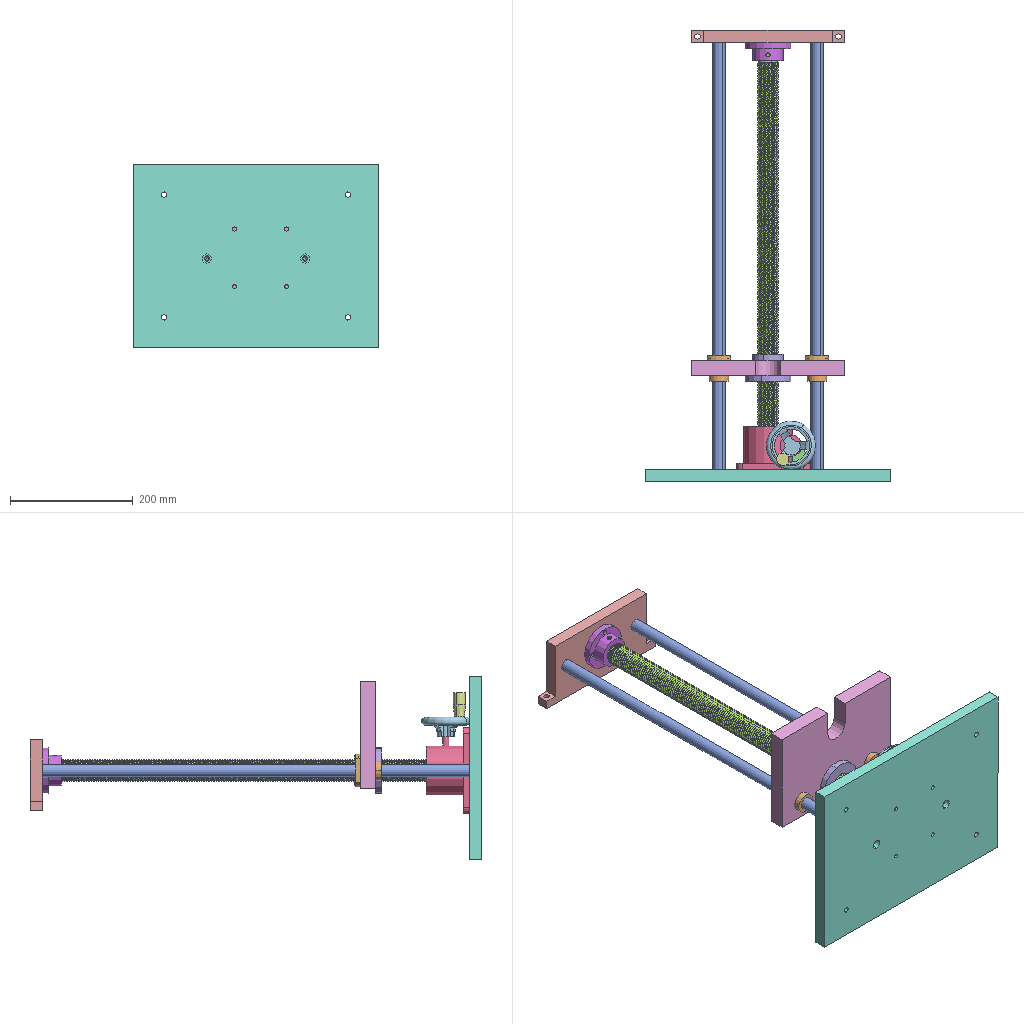Assembly | SolidWorks | 12 different items | 14 placed | box 400 x 736 x 300 mm
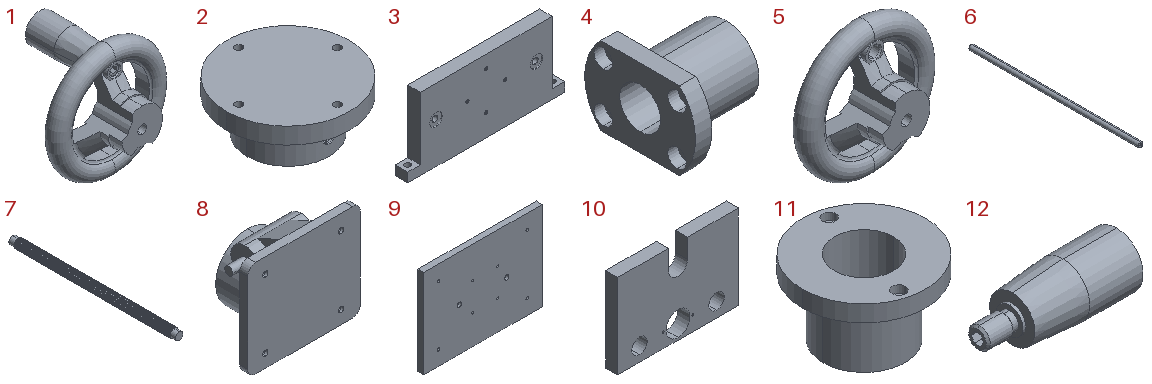Parts list (item | name | quantity | parent item | size | volume | features):
1 | (subassembly) | x1 | - | 80 x 72 x 80 mm | 60267 mm3 | -
2 | - | x1 | - | 75 x 75 x 30 mm | 67720 mm3 | features HoleWzd 2, ICE 2, 3DProfileFeature 1, CirPattern 1, Extrusion 1, SweepThread 1
3 | - | x1 | - | 250 x 20 x 115 mm | 486183 mm3 | features SweepThread 4, HoleWzd 3, Extrusion 1, ICE 1, MirrorPattern 1
4 | - | x2 | - | 42 x 54 x 38 mm | 27513 mm3 | features BaseBody 1
5 | - | x1 | in 1 | 80 x 32 x 80 mm | 48291 mm3 | features RefAxis 9, 3DProfileFeature 3, Revolution 3, RevCut 2, CirPattern 1, ICE 1
6 | - | x2 | - | 20 x 700 x 20 mm | 218428 mm3 | features HoleWzd 2, Extrusion 1
7 | - | x1 | - | 36 x 670 x 36 mm | 568106 mm3 | features ICE 2, Extrusion 1, SweepThread 1
8 | - | x1 | - | 140 x 70 x 120 mm | 525690 mm3 | features ICE 4, Extrusion 1, Fillet 1, HoleWzd 1
9 | - | x1 | - | 400 x 20 x 300 mm | 2382351 mm3 | features HoleWzd 3, Cut 1, Extrusion 1
10 | - | x1 | - | 250 x 25 x 175 mm | 946629 mm3 | features ICE 3, HoleWzd 2, Extrusion 1, MirrorPattern 1
11 | - | x1 | - | 75 x 75 x 45 mm | 66462 mm3 | features Extrusion 1, HoleWzd 1, ICE 1
12 | - | x1 | in 1 | 52 x 20 x 20 mm | 11976 mm3 | features RefAxis 3, 3DProfileFeature 1, ICE 1, RevCut 1, Revolution 1
Mates (type | each side: item.copy, entity, surface, feature):
Concentric | 3.1 face cylinder Hole size per socket head cap screw type1 | 6.1 face cylinder Boss-Extrude1
Concentric | 3.1 face cylinder Hole size per socket head cap screw type1 | 6.2 face cylinder Boss-Extrude1
Coincident | 3.1 face plane Cut-Extrude1 | 6.1 face plane Boss-Extrude1
Coincident | 3.1 face plane Cut-Extrude1 | 6.2 face plane Boss-Extrude1
Width | 10.1 face plane Boss-Extrude1 | 10.1 face plane Boss-Extrude1 | 3.1 face plane Boss-Extrude1 | 3.1 face plane Boss-Extrude1
Concentric | 6.1 face cylinder Boss-Extrude1 | 10.1 face cylinder Cut-Extrude2
Concentric | 6.2 face cylinder Boss-Extrude1 | 10.1 face cylinder Cut-Extrude2
Concentric | 7.1 face cylinder Boss-Extrude1 | 10.1 face cylinder Cut-Extrude3
Width | 9.1 face plane Boss-Extrude1 | 9.1 face plane Boss-Extrude1 | 10.1 face plane Boss-Extrude1 | 10.1 face plane Boss-Extrude1
Coincident | 6.1 face plane Boss-Extrude1 | 9.1 face plane Cut-Extrude1
Concentric | 6.1 face cylinder Boss-Extrude1 | 4.1 face cylinder Input1
Parallel | 10.1 face plane Boss-Extrude1 | 4.1 face plane Input1
Coincident | 10.1 face plane Boss-Extrude1 | 4.1 face plane Input1
Concentric | 6.2 face cylinder Boss-Extrude1 | 4.2 face cylinder Input1
Parallel | 4.1 face plane Input1 | 4.2 face plane Input1
Coincident | 10.1 face plane Boss-Extrude1 | 4.2 face plane Input1
Concentric | 7.1 face cylinder Boss-Extrude1 | 11.1 face cylinder Boss-Extrude1
Coincident | 10.1 face plane Boss-Extrude1 | 11.1 face plane Boss-Extrude2
Concentric | 11.1 face cylinder Boss-Extrude1 | 8.1 face cylinder Boss-Extrude1
Coincident | 9.1 face plane Boss-Extrude1 | 8.1 face plane Boss-Extrude2
Parallel | 9.1 face plane Boss-Extrude1 | 8.1 face plane Boss-Extrude2
Concentric | 8.1 face cylinder Boss-Extrude7 | 5.1 face cylinder CirPattern1
DistanceDim | 8.1 face plane Boss-Extrude3 | 5.1 face plane Revolve2
Concentric | 7.1 face cylinder Boss-Extrude1 | 2.1 face cylinder Boss-Extrude1
Coincident | 7.1 face plane Boss-Extrude1 | 2.1 face plane Boss-Extrude2
Coincident | 3.1 face plane Boss-Extrude1 | 2.1 face plane Boss-Extrude2
Parallel | 3.1 face plane Boss-Extrude1 | 2.1 plane